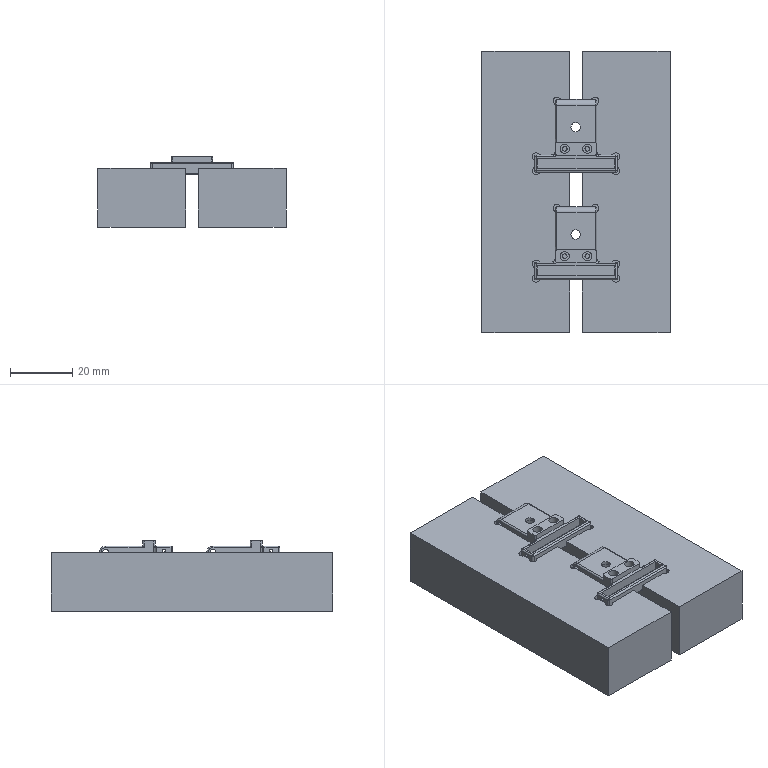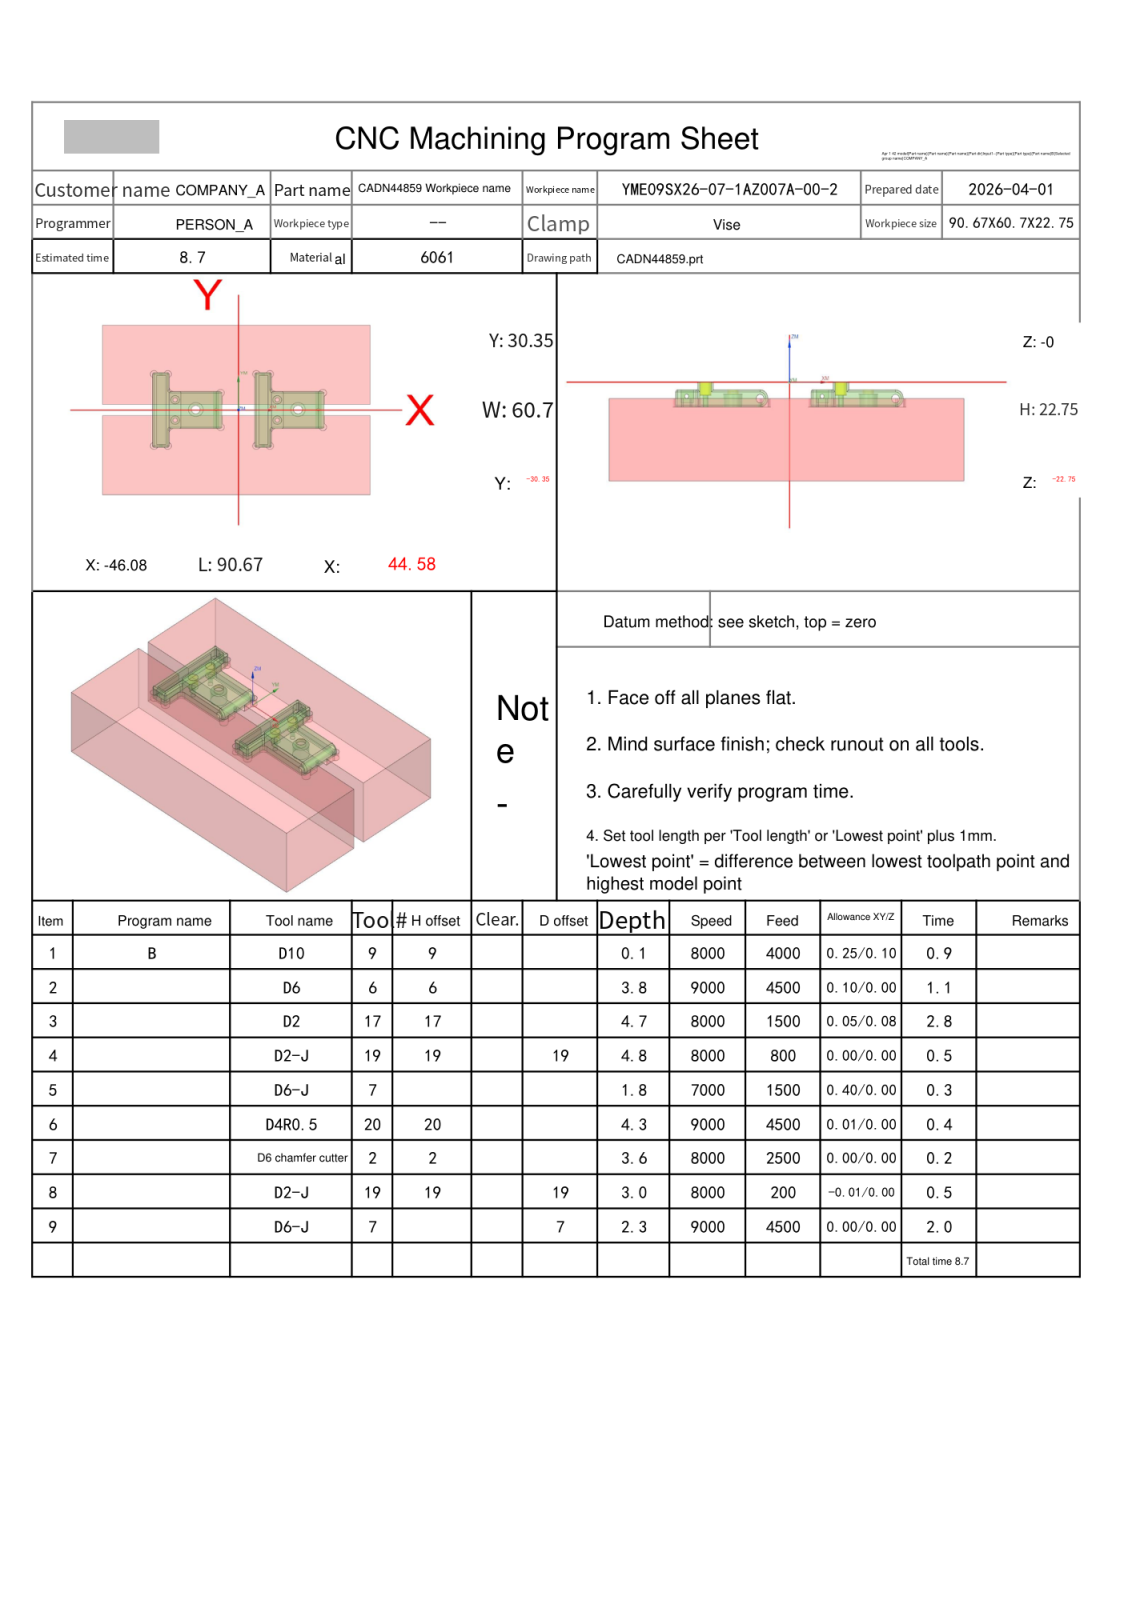NC program | NX | posted by the shop | part box 60.696 x 90.669 x 22.754 mm
Lines 3625 to 6042 of 6042, first 1914 of 2418 lines:
N7 T02 M06
(D6 chamfer cutter  D=6. R=0. H=02 ce=0.00 di=0.00)
G00 G90 G54 X-21.452 Y3.634 M03 S8000
G43 H02 Z20.
M08
G98 G82 X-21.452 Y3.634 Z-1. R1. F2500.
Y-3.634
X13.148
Y3.634
G80
G00 Z20.
G00 G90 X-14.452 Y.15 M03 S8000
Z20.
G98 G81 X-14.452 Y.15 Z-3.554 R1.246 F1000.
X20.148
G80
G00 Z20.
G00 G90 X-21.452 Y3.634 M03 S8000
Z20.
G98 G81 X-21.452 Y3.634 Z-1.8 R3. F1000.
Y-3.634
X13.148
Y3.634
G80
G00 Z20.
G00 G90 X10.121 Y-.386 M03 S6500
Z20.
Z.372
G01 Z-.999 F1500.
G03 X10.321 Y-.1 I-1.532 J1.286
G01 X10.351 Y-.054
X10.348 Y0.0
Y6.134
G02 X11.648 Y7.434 I1.3 J0.0
G01 X14.648
G02 X15.948 Y6.134 I0.0 J-1.3
G01 Y-6.134
G02 X14.648 Y-7.434 I-1.3 J0.0
G01 X11.648
G02 X10.348 Y-6.134 I0.0 J1.3
G01 Y0.0
X10.351 Y.054
X10.321 Y.1
G03 X10.121 Y.386 I-1.732 J-1.
G01 Z.372
G00 Z2.751
X12.736 Y3.108
Z.572
G01 Z-.999
G03 X13.045 Y2.947 I1.075 J1.687
G01 X13.094 Y2.924
X13.148 Y2.934
G03 X13.848 Y3.634 I0.0 J.7
X13.148 Y4.334 I-.7 J0.0
X12.448 Y3.634 I0.0 J-.7
X12.967 Y2.958 I.7 J0.0
G01 X13.148 Y2.934
X13.201 Y2.924
X13.25 Y2.947
G03 X13.56 Y3.108 I-.765 J1.848
G01 Z.572
G00 Z2.751
X12.736 Y-4.159
Z.572
G01 Z-.999
G03 X13.045 Y-4.32 I1.075 J1.687
G01 X13.094 Y-4.344
X13.148 Y-4.334
G03 X13.848 Y-3.634 I0.0 J.7
X13.148 Y-2.934 I-.7 J0.0
X12.448 Y-3.634 I0.0 J-.7
X12.967 Y-4.31 I.7 J0.0
G01 X13.148 Y-4.334
X13.201 Y-4.344
X13.25 Y-4.32
G03 X13.56 Y-4.159 I-.765 J1.848
G01 Z.572
G00 Z10.
X-18.426 Y.386
Z.372
G01 Z-.999
G03 X-18.625 Y.1 I1.532 J-1.286
G01 X-18.655 Y.054
X-18.652 Y0.0
Y-6.134
G02 X-19.952 Y-7.434 I-1.3 J0.0
G01 X-22.952
G02 X-24.252 Y-6.134 I0.0 J1.3
G01 Y6.134
G02 X-22.952 Y7.434 I1.3 J0.0
G01 X-19.952
G02 X-18.652 Y6.134 I0.0 J-1.3
G01 Y0.0
X-18.655 Y-.054
X-18.625 Y-.1
G03 X-18.426 Y-.386 I1.732 J1.
G01 Z.372
G00 Z2.751
X-21.864 Y3.108
Z.572
G01 Z-.999
G03 X-21.555 Y2.947 I1.075 J1.687
G01 X-21.506 Y2.924
X-21.452 Y2.934
G03 X-20.752 Y3.634 I0.0 J.7
X-21.452 Y4.334 I-.7 J0.0
X-22.152 Y3.634 I0.0 J-.7
X-21.633 Y2.958 I.7 J0.0
G01 X-21.452 Y2.934
X-21.399 Y2.924
X-21.35 Y2.947
G03 X-21.04 Y3.108 I-.765 J1.848
G01 Z.572
G00 Z2.751
X-21.864 Y-4.159
Z.572
G01 Z-.999
G03 X-21.555 Y-4.32 I1.075 J1.687
G01 X-21.506 Y-4.344
X-21.452 Y-4.334
G03 X-20.752 Y-3.634 I0.0 J.7
X-21.452 Y-2.934 I-.7 J0.0
X-22.152 Y-3.634 I0.0 J-.7
X-21.633 Y-4.31 I.7 J0.0
G01 X-21.452 Y-4.334
X-21.399 Y-4.344
X-21.35 Y-4.32
G03 X-21.04 Y-4.159 I-.765 J1.848
G01 Z.572
G00 Z10.
X-25.344 Y8.3
Z1.247
G01 Z-2.753
Y11.548
X-26.896
Y-11.548
X-25.344
Y-8.3
Z1.247
G00 Z10.
X-14.864 Y-.376
Z-1.182
G01 Z-2.753
G03 X-14.555 Y-.536 I1.075 J1.687
G01 X-14.506 Y-.56
X-14.452 Y-.55
G03 X-13.752 Y.15 I0.0 J.7
X-14.452 Y.85 I-.7 J0.0
X-15.152 Y.15 I0.0 J-.7
X-14.633 Y-.526 I.7 J0.0
G01 X-14.452 Y-.55
X-14.399 Y-.56
X-14.35 Y-.536
G03 X-14.04 Y-.376 I-.765 J1.848
G01 Z-1.182
G00 Z10.
X9.256 Y8.3
Z1.247
G01 Z-2.753
Y11.548
X7.704
Y0.0
Y-11.548
X9.256
Y-8.3
Z1.247
G00 Z10.
X19.736 Y-.376
Z-1.182
G01 Z-2.753
G03 X20.045 Y-.536 I1.075 J1.687
G01 X20.094 Y-.56
X20.148 Y-.55
G03 X20.848 Y.15 I0.0 J.7
X20.148 Y.85 I-.7 J0.0
X19.448 Y.15 I0.0 J-.7
X19.967 Y-.526 I.7 J0.0
G01 X20.148 Y-.55
X20.201 Y-.56
X20.25 Y-.536
G03 X20.56 Y-.376 I-.765 J1.848
G01 Z-1.182
G00 Z20.
G91 G28 Z0.0
M05
M09
G91 G28 Z0.0
M01
N8 T19 M06
(D2-J  D=2. R=0. H=19 ce=-0.01 di=0.00)
G00 G90 G54 X12.716 Y-3.825 M03 S8000
G43 H19 Z20.
M08
Z.5
G01 X12.737 Y-3.884 Z.497 F200.
X12.868 Y-4.025 Z.487
X13.043 Y-4.103 Z.477
X13.217 Y-4.11 Z.467
X13.363 Y-4.064 Z.459
X13.488 Y-3.974 Z.451
X13.578 Y-3.849 Z.443
X13.624 Y-3.703 Z.435
Y-3.565 Z.428
X13.578 Y-3.418 Z.42
X13.488 Y-3.294 Z.412
X13.363 Y-3.204 Z.404
X13.217 Y-3.158 Z.396
X13.079 Z.389
X12.932 Y-3.204 Z.381
X12.808 Y-3.294 Z.372
X12.718 Y-3.418 Z.364
X12.672 Y-3.565 Z.356
Y-3.703 Z.349
X12.737 Y-3.884 Z.339
X12.868 Y-4.025 Z.329
X13.043 Y-4.103 Z.319
X13.217 Y-4.11 Z.31
X13.363 Y-4.064 Z.302
X13.488 Y-3.974 Z.294
X13.578 Y-3.849 Z.286
X13.624 Y-3.703 Z.278
Y-3.565 Z.27
X13.578 Y-3.418 Z.262
X13.488 Y-3.294 Z.254
X13.363 Y-3.204 Z.246
X13.217 Y-3.158 Z.238
X13.079 Z.231
X12.932 Y-3.204 Z.223
X12.808 Y-3.294 Z.215
X12.718 Y-3.418 Z.207
X12.672 Y-3.565 Z.199
Y-3.703 Z.191
X12.737 Y-3.884 Z.181
X12.868 Y-4.025 Z.171
X13.043 Y-4.103 Z.161
X13.217 Y-4.11 Z.152
X13.363 Y-4.064 Z.144
X13.488 Y-3.974 Z.136
X13.578 Y-3.849 Z.128
X13.624 Y-3.703 Z.12
Y-3.565 Z.113
X13.578 Y-3.418 Z.105
X13.488 Y-3.294 Z.097
X13.363 Y-3.204 Z.089
X13.217 Y-3.158 Z.081
X13.079 Z.073
X12.932 Y-3.204 Z.065
X12.808 Y-3.294 Z.057
X12.718 Y-3.418 Z.049
X12.672 Y-3.565 Z.041
Y-3.703 Z.034
X12.737 Y-3.884 Z.024
X12.868 Y-4.025 Z.014
X13.043 Y-4.103 Z.004
X13.112 Y-4.108 Z0.0
G41 D19
X13.148 Y-4.144
G03 X13.658 Y-3.634 Z-.25 I0.0 J.51
X13.148 Y-3.124 Z-.5 I-.51 J0.0
X12.638 Y-3.634 Z-.75 I0.0 J-.51
X13.148 Y-4.144 Z-1. I.51 J0.0
X13.658 Y-3.634 Z-1.25 I0.0 J.51
X13.148 Y-3.124 Z-1.5 I-.51 J0.0
X12.638 Y-3.634 Z-1.75 I0.0 J-.51
X13.148 Y-4.144 Z-2. I.51 J0.0
X13.658 Y-3.634 Z-2.25 I0.0 J.51
X13.148 Y-3.124 Z-2.5 I-.51 J0.0
X12.638 Y-3.634 Z-2.75 I0.0 J-.51
X13.148 Y-4.144 Z-3. I.51 J0.0
X13.658 Y-3.634 I0.0 J.51
X13.148 Y-3.124 I-.51 J0.0
X12.638 Y-3.634 I0.0 J-.51
X13.148 Y-4.144 I.51 J0.0
X13.508 Y-3.995 I0.0 J.51
G01 X13.526 Y-3.974
Y-3.945
X13.508 Y-3.924
G40 X13.473 Y-3.889
Z-2.
G00 Z20.
X13.58 Y3.825
Z.5
G01 X13.559 Y3.884 Z.497
X13.428 Y4.025 Z.487
X13.252 Y4.103 Z.477
X13.079 Y4.11 Z.467
X12.932 Y4.064 Z.459
X12.808 Y3.974 Z.451
X12.718 Y3.849 Z.443
X12.672 Y3.703 Z.435
Y3.565 Z.428
X12.718 Y3.418 Z.42
X12.808 Y3.294 Z.412
X12.932 Y3.204 Z.404
X13.079 Y3.158 Z.396
X13.217 Z.389
X13.363 Y3.204 Z.381
X13.488 Y3.294 Z.372
X13.578 Y3.418 Z.364
X13.624 Y3.565 Z.356
Y3.703 Z.349
X13.559 Y3.884 Z.339
X13.428 Y4.025 Z.329
X13.252 Y4.103 Z.319
X13.079 Y4.11 Z.31
X12.932 Y4.064 Z.302
X12.808 Y3.974 Z.294
X12.718 Y3.849 Z.286
X12.672 Y3.703 Z.278
Y3.565 Z.27
X12.718 Y3.418 Z.262
X12.808 Y3.294 Z.254
X12.932 Y3.204 Z.246
X13.079 Y3.158 Z.238
X13.217 Z.231
X13.363 Y3.204 Z.223
X13.488 Y3.294 Z.215
X13.578 Y3.418 Z.207
X13.624 Y3.565 Z.199
Y3.703 Z.191
X13.559 Y3.884 Z.181
X13.428 Y4.025 Z.171
X13.252 Y4.103 Z.161
X13.079 Y4.11 Z.152
X12.932 Y4.064 Z.144
X12.808 Y3.974 Z.136
X12.718 Y3.849 Z.128
X12.672 Y3.703 Z.12
Y3.565 Z.113
X12.718 Y3.418 Z.105
X12.808 Y3.294 Z.097
X12.932 Y3.204 Z.089
X13.079 Y3.158 Z.081
X13.217 Z.073
X13.363 Y3.204 Z.065
X13.488 Y3.294 Z.057
X13.578 Y3.418 Z.049
X13.624 Y3.565 Z.041
Y3.703 Z.034
X13.559 Y3.884 Z.024
X13.428 Y4.025 Z.014
X13.252 Y4.103 Z.004
X13.183 Y4.108 Z0.0
G41 D19
X13.148 Y4.144
G03 X12.638 Y3.634 Z-.25 I0.0 J-.51
X13.148 Y3.124 Z-.5 I.51 J0.0
X13.658 Y3.634 Z-.75 I0.0 J.51
X13.148 Y4.144 Z-1. I-.51 J0.0
X12.638 Y3.634 Z-1.25 I0.0 J-.51
X13.148 Y3.124 Z-1.5 I.51 J0.0
X13.658 Y3.634 Z-1.75 I0.0 J.51
X13.148 Y4.144 Z-2. I-.51 J0.0
X12.638 Y3.634 Z-2.25 I0.0 J-.51
X13.148 Y3.124 Z-2.5 I.51 J0.0
X13.658 Y3.634 Z-2.75 I0.0 J.51
X13.148 Y4.144 Z-3. I-.51 J0.0
X12.638 Y3.634 I0.0 J-.51
X13.148 Y3.124 I.51 J0.0
X13.658 Y3.634 I0.0 J.51
X13.148 Y4.144 I-.51 J0.0
X12.787 Y3.995 I0.0 J-.51
G01 X12.77 Y3.974
Y3.945
X12.787 Y3.924
G40 X12.823 Y3.889
Z-2.
G00 Z20.
X-21.643 Y4.066
Z.5
G01 X-21.702 Y4.045 Z.497
X-21.843 Y3.914 Z.487
X-21.922 Y3.738 Z.477
X-21.928 Y3.565 Z.467
X-21.882 Y3.418 Z.459
X-21.792 Y3.294 Z.451
X-21.668 Y3.204 Z.443
X-21.521 Y3.158 Z.435
X-21.383 Z.428
X-21.237 Y3.204 Z.42
X-21.112 Y3.294 Z.412
X-21.022 Y3.418 Z.404
X-20.976 Y3.565 Z.396
Y3.703 Z.389
X-21.022 Y3.849 Z.381
X-21.112 Y3.974 Z.372
X-21.237 Y4.064 Z.364
X-21.383 Y4.11 Z.356
X-21.521 Z.349
X-21.702 Y4.045 Z.339
X-21.843 Y3.914 Z.329
X-21.922 Y3.738 Z.319
X-21.928 Y3.565 Z.31
X-21.882 Y3.418 Z.302
X-21.792 Y3.294 Z.294
X-21.668 Y3.204 Z.286
X-21.521 Y3.158 Z.278
X-21.383 Z.27
X-21.237 Y3.204 Z.262
X-21.112 Y3.294 Z.254
X-21.022 Y3.418 Z.246
X-20.976 Y3.565 Z.238
Y3.703 Z.231
X-21.022 Y3.849 Z.223
X-21.112 Y3.974 Z.215
X-21.237 Y4.064 Z.207
X-21.383 Y4.11 Z.199
X-21.521 Z.191
X-21.702 Y4.045 Z.181
X-21.843 Y3.914 Z.171
X-21.922 Y3.738 Z.161
X-21.928 Y3.565 Z.152
X-21.882 Y3.418 Z.144
X-21.792 Y3.294 Z.136
X-21.668 Y3.204 Z.128
X-21.521 Y3.158 Z.12
X-21.383 Z.113
X-21.237 Y3.204 Z.105
X-21.112 Y3.294 Z.097
X-21.022 Y3.418 Z.089
X-20.976 Y3.565 Z.081
Y3.703 Z.073
X-21.022 Y3.849 Z.065
X-21.112 Y3.974 Z.057
X-21.237 Y4.064 Z.049
X-21.383 Y4.11 Z.041
X-21.521 Z.034
X-21.702 Y4.045 Z.024
X-21.843 Y3.914 Z.014
X-21.922 Y3.738 Z.004
X-21.927 Y3.669 Z0.0
G41 D19
X-21.962 Y3.634
G03 X-21.452 Y3.124 Z-.25 I.51 J0.0
X-20.942 Y3.634 Z-.5 I0.0 J.51
X-21.452 Y4.144 Z-.75 I-.51 J0.0
X-21.962 Y3.634 Z-1. I0.0 J-.51
X-21.452 Y3.124 Z-1.25 I.51 J0.0
X-20.942 Y3.634 Z-1.5 I0.0 J.51
X-21.452 Y4.144 Z-1.75 I-.51 J0.0
X-21.962 Y3.634 Z-2. I0.0 J-.51
X-21.452 Y3.124 Z-2.25 I.51 J0.0
X-20.942 Y3.634 Z-2.5 I0.0 J.51
X-21.452 Y4.144 Z-2.75 I-.51 J0.0
X-21.962 Y3.634 Z-3. I0.0 J-.51
X-21.452 Y3.124 I.51 J0.0
X-20.942 Y3.634 I0.0 J.51
X-21.452 Y4.144 I-.51 J0.0
X-21.962 Y3.634 I0.0 J-.51
X-21.813 Y3.274 I.51 J0.0
G01 X-21.792 Y3.256
X-21.764
X-21.743 Y3.274
G40 X-21.707 Y3.309
Z-2.
G00 Z20.
X-21.643 Y-3.202
Z.5
G01 X-21.702 Y-3.223 Z.497
X-21.843 Y-3.354 Z.487
X-21.922 Y-3.53 Z.477
X-21.928 Y-3.703 Z.467
X-21.882 Y-3.849 Z.459
X-21.792 Y-3.974 Z.451
X-21.668 Y-4.064 Z.443
X-21.521 Y-4.11 Z.435
X-21.383 Z.428
X-21.237 Y-4.064 Z.42
X-21.112 Y-3.974 Z.412
X-21.022 Y-3.849 Z.404
X-20.976 Y-3.703 Z.396
Y-3.565 Z.389
X-21.022 Y-3.418 Z.381
X-21.112 Y-3.294 Z.372
X-21.237 Y-3.204 Z.364
X-21.383 Y-3.158 Z.356
X-21.521 Z.349
X-21.702 Y-3.223 Z.339
X-21.843 Y-3.354 Z.329
X-21.922 Y-3.53 Z.319
X-21.928 Y-3.703 Z.31
X-21.882 Y-3.849 Z.302
X-21.792 Y-3.974 Z.294
X-21.668 Y-4.064 Z.286
X-21.521 Y-4.11 Z.278
X-21.383 Z.27
X-21.237 Y-4.064 Z.262
X-21.112 Y-3.974 Z.254
X-21.022 Y-3.849 Z.246
X-20.976 Y-3.703 Z.238
Y-3.565 Z.231
X-21.022 Y-3.418 Z.223
X-21.112 Y-3.294 Z.215
X-21.237 Y-3.204 Z.207
X-21.383 Y-3.158 Z.199
X-21.521 Z.191
X-21.702 Y-3.223 Z.181
X-21.843 Y-3.354 Z.171
X-21.922 Y-3.53 Z.161
X-21.928 Y-3.703 Z.152
X-21.882 Y-3.849 Z.144
X-21.792 Y-3.974 Z.136
X-21.668 Y-4.064 Z.128
X-21.521 Y-4.11 Z.12
X-21.383 Z.113
X-21.237 Y-4.064 Z.105
X-21.112 Y-3.974 Z.097
X-21.022 Y-3.849 Z.089
X-20.976 Y-3.703 Z.081
Y-3.565 Z.073
X-21.022 Y-3.418 Z.065
X-21.112 Y-3.294 Z.057
X-21.237 Y-3.204 Z.049
X-21.383 Y-3.158 Z.041
X-21.521 Z.034
X-21.702 Y-3.223 Z.024
X-21.843 Y-3.354 Z.014
X-21.922 Y-3.53 Z.004
X-21.927 Y-3.598 Z0.0
G41 D19
X-21.962 Y-3.634
G03 X-21.452 Y-4.144 Z-.25 I.51 J0.0
X-20.942 Y-3.634 Z-.5 I0.0 J.51
X-21.452 Y-3.124 Z-.75 I-.51 J0.0
X-21.962 Y-3.634 Z-1. I0.0 J-.51
X-21.452 Y-4.144 Z-1.25 I.51 J0.0
X-20.942 Y-3.634 Z-1.5 I0.0 J.51
X-21.452 Y-3.124 Z-1.75 I-.51 J0.0
X-21.962 Y-3.634 Z-2. I0.0 J-.51
X-21.452 Y-4.144 Z-2.25 I.51 J0.0
X-20.942 Y-3.634 Z-2.5 I0.0 J.51
X-21.452 Y-3.124 Z-2.75 I-.51 J0.0
X-21.962 Y-3.634 Z-3. I0.0 J-.51
X-21.452 Y-4.144 I.51 J0.0
X-20.942 Y-3.634 I0.0 J.51
X-21.452 Y-3.124 I-.51 J0.0
X-21.962 Y-3.634 I0.0 J-.51
X-21.813 Y-3.994 I.51 J0.0
G01 X-21.792 Y-4.012
X-21.764
X-21.743 Y-3.994
G40 X-21.707 Y-3.959
Z-2.
G00 Z20.
G91 G28 Z0.0
M05
M09
G91 G28 Z0.0
M01
N9 T07 M06
(D6-J  D=6. R=0. H=00 ce=0.00 di=0.00)
G00 G90 G54 X13.748 Y10.734 M03 S8000
G43 H00 Z6.95
M08
Z-.754
G01 Z-1.754 F1000.
G41 D07
Y10.534
G03 X14.648 Y9.634 I.9 J0.0
G02 X18.148 Y6.134 I0.0 J-3.5
G01 Y6.131
Y-6.129
Y-6.134
G02 X14.648 Y-9.634 I-3.5 J0.0
G03 X13.748 Y-10.534 I0.0 J-.9
G01 G40 Y-10.734
Z-.754
G00 Z6.95
X12.548
Z-.754
G01 Z-1.754
G41 D07
Y-10.534
G03 X11.648 Y-9.634 I-.9 J0.0
G02 X8.148 Y-6.134 I0.0 J3.5
G01 Y6.134
G02 X11.648 Y9.634 I3.5 J0.0
G03 X12.548 Y10.534 I0.0 J.9
G01 G40 Y10.734
Z-.754
G00 Z6.95
X-20.852
Z-.754
G01 Z-1.754
G41 D07
Y10.534
G03 X-19.952 Y9.634 I.9 J0.0
G02 X-16.452 Y6.134 I0.0 J-3.5
G01 Y6.131
Y-6.129
Y-6.134
G02 X-19.952 Y-9.634 I-3.5 J0.0
G03 X-20.852 Y-10.534 I0.0 J-.9
G01 G40 Y-10.734
Z-.754
G00 Z6.95
X-22.052
Z-.754
G01 Z-1.754
G41 D07
Y-10.534
G03 X-22.952 Y-9.634 I-.9 J0.0
G02 X-26.452 Y-6.134 I0.0 J3.5
G01 Y6.134
G02 X-22.952 Y9.634 I3.5 J0.0
G03 X-22.052 Y10.534 I0.0 J.9
G01 G40 Y10.734
Z-.754
G00 Z6.95
G00 G90 X-3.703 Y-11.541 M03 S9000
Z11.95
Z-1.262
G01 Z-1.762 F4500.
G03 X-6.415 Y-9.176 I-2.934 J-.627
X-6.741 Y-9.164 I-.326 J-4.399
X-7.515 Y-9.233 I0.0 J-4.411
G01 X-18.304
X-18.342 Y-9.253 Z-1.766
X-7.515
G02 X-6.724 Y-9.189 I.792 J-4.853
X-6.415 Y-9.198 I0.0 J-4.917
G01 X-6.414 Y-9.221 Z-1.77
G03 X-6.696 Y-9.214 I-.282 J-6.068
X-7.515 Y-9.27 I0.0 J-6.074
G01 X-18.375
X-18.405 Y-9.285 Z-1.774
X-7.515
G02 X-6.672 Y-9.239 I.844 J-7.802
X-6.414 Y-9.243 I0.0 J-7.848
G01 X-6.413 Y-9.27 Z-1.779
G03 X-7.515 Y-9.3 I1.192 J-63.284
G01 X-18.437
X-18.467 Y-9.314 Z-1.784
X-7.515
X-6.412 Y-9.296
X-6.414 Y-9.312 Z-1.787
Y-9.313 Z-1.789
X-6.6
G03 X-7.515 Y-9.329 I0.0 J-26.271
G01 X-18.499
X-18.53 Y-9.343 Z-1.795
X-7.515
G02 X-6.603 Y-9.325 I.913 J-23.879
G01 X-6.414 Y-9.326
Y-9.338 Z-1.798
Y-9.34 Z-1.802
G03 X-7.515 Y-9.357 I.605 J-74.86
G01 X-18.561
X-18.594 Y-9.37 Z-1.808
X-7.515
G02 X-6.413 Y-9.354 I5.167 J-313.246
G01 Y-9.368 Z-1.812
Y-9.369 Z-1.815
X-7.515 Y-9.384
X-18.626
X-18.658 Y-9.397 Z-1.823
X-7.515
X-6.413 Y-9.385
X-6.414 Y-9.396 Z-1.827
Y-9.398 Z-1.831
X-7.515 Y-9.41
X-18.692
X-18.725 Y-9.422 Z-1.839
X-7.515
G02 X-6.549 Y-9.409 I.966 J-35.239
G01 X-6.414
Y-9.42 Z-1.843
Y-9.421 Z-1.847
X-6.547
G03 X-7.515 Y-9.435 I0.0 J-33.728
G01 X-18.759
X-18.777 Y-9.441 Z-1.856
X-7.515
G02 X-6.539 Y-9.427 I.977 J-34.327
G01 X-6.415
Y-9.445 Z-1.861
Y-9.446 Z-1.866
X-7.515 Y-9.459
X-18.828
X-18.859 Y-9.469 Z-1.875
X-7.515
X-6.415 Y-9.458
X-6.416 Y-9.47 Z-1.881
Y-9.473 Z-1.886
X-7.515 Y-9.482
X-18.898
X-18.934 Y-9.493 Z-1.896
X-7.515
X-6.414 Y-9.486
Y-9.495 Z-1.907
X-7.515 Y-9.503
X-18.969
X-19.006 Y-9.514 Z-1.918
X-7.515
G02 X-6.723 Y-9.504 I.793 J-30.792
X-6.414 Y-9.505 I0.0 J-30.803
G01 Y-9.513 Z-1.929
G03 X-6.725 Y-9.511 I-.311 J-30.346
X-7.515 Y-9.522 I0.0 J-30.347
G01 X-19.034
X-19.079 Y-9.533 Z-1.941
X-7.515
G02 X-6.728 Y-9.524 I.787 J-32.489
X-6.414 Y-9.525 I0.0 J-32.498
G01 Y-9.532 Z-1.947
Y-9.536 Z-1.952
X-7.515 Y-9.543
X-19.116
X-19.153 Y-9.552 Z-1.965
X-7.515
X-6.414 Y-9.547
Y-9.548 Z-1.971
Y-9.557 Z-1.977
X-7.515 Y-9.56
X-19.19
X-19.228 Y-9.568 Z-1.99
X-7.515
X-6.414 Y-9.565
Y-9.572 Z-2.003
X-7.515 Y-9.576
X-19.266
X-19.304 Y-9.583 Z-2.016
X-7.515
X-6.414 Y-9.579
Y-9.586 Z-2.029
X-7.515 Y-9.59
X-19.342
X-19.381 Y-9.597 Z-2.043
X-7.515
X-6.414 Y-9.593
Y-9.6 Z-2.056
X-7.515 Y-9.603
X-19.419
X-19.458 Y-9.609 Z-2.07
X-7.515
X-6.414 Y-9.603
Y-9.607 Z-2.084
X-7.515 Y-9.614
X-19.497
X-19.536 Y-9.619 Z-2.099
X-7.515
X-6.414 Y-9.611
Y-9.614 Z-2.113
X-7.515 Y-9.624
X-19.576
X-19.615 Y-9.628 Z-2.128
X-7.515
X-6.42 Y-9.617
X-6.414 Y-9.618
Y-9.622 Z-2.142
X-6.42 Y-9.62
X-7.515 Y-9.631
X-19.654
X-19.694 Y-9.634 Z-2.157
X-7.515
X-6.42 Y-9.623
X-6.414 Y-9.626
Y-9.63 Z-2.172
X-6.42 Y-9.627
X-7.515 Y-9.637
X-19.733
X-19.773 Y-9.639 Z-2.186
X-7.515
X-6.42 Y-9.63
X-6.414 Y-9.633
Y-9.635 Z-2.201
X-7.515 Y-9.641
X-19.813
X-19.852 Y-9.642 Z-2.216
X-7.515
X-6.42 Y-9.637
X-6.414 Y-9.638
Y-9.641 Z-2.231
X-19.852 Y-9.643
X-19.892
X-20.03 Y-9.644 Z-2.237
X-20.169 Z-2.243
X-20.31 Z-2.248
X-20.442 Y-9.654 Z-2.254
X-20.432 Y-9.644
X-19.93
X-19.87 Y-9.643
X-6.414
G00 Z11.95
X-15.305 Y12.233
Z-1.262
G01 Z-1.762
G03 X-18.304 Y9.233 I0.0 J-3.
G01 X-7.515
X-6.863 Y9.178
X-6.418 Y9.186
X-6.419 Y9.208 Z-1.766
X-6.863 Y9.2
G03 X-7.515 Y9.253 I-.86 J-6.625
G01 X-18.342
X-18.375 Y9.27 Z-1.77
X-7.515
G03 X-6.627 Y9.226 I.889 J9.11
X-6.418 Y9.229 I0.0 J9.153
G01 X-6.417 Y9.25 Z-1.774
G02 X-6.631 Y9.248 I-.213 J10.606
X-7.515 Y9.285 I0.0 J10.608
G01 X-18.405
X-18.437 Y9.3 Z-1.779
X-7.515
X-6.416 Y9.274
X-6.414 Y9.295 Z-1.781
X-6.413 Y9.299 Z-1.784
X-7.515 Y9.314
X-18.467
X-18.499 Y9.329 Z-1.789
X-7.515
G03 X-6.6 Y9.313 I.916 J26.601
G01 X-6.414 Y9.314
Y9.323 Z-1.792
Y9.326 Z-1.795
X-6.604 Y9.325
G02 X-7.515 Y9.343 I0.0 J23.966
G01 X-18.53
X-18.561 Y9.357 Z-1.802
X-7.515
G03 X-6.593 Y9.339 I.923 J24.065
G01 X-6.414 Y9.34
X-6.413 Y9.352 Z-1.805
Y9.354 Z-1.808
X-6.563
G02 X-7.515 Y9.37 I0.0 J27.089
G01 X-18.594
X-18.626 Y9.384 Z-1.815
X-7.515
X-6.413 Y9.369
Y9.382 Z-1.819
Y9.385 Z-1.823
X-7.515 Y9.397
X-18.658
X-18.692 Y9.41 Z-1.831
X-7.515
G03 X-6.534 Y9.398 I.981 J40.461
G01 X-6.414
Y9.407 Z-1.835
Y9.409 Z-1.839
X-6.553
G02 X-7.515 Y9.422 I0.0 J34.718
G01 X-18.725
X-18.759 Y9.435 Z-1.847
X-7.515
G03 X-6.548 Y9.421 I.967 J33.574
G01 X-6.414
X-6.415 Y9.427 Z-1.856
X-6.539
G02 X-7.515 Y9.441 I0.0 J34.388
G01 X-18.777
X-18.828 Y9.459 Z-1.866
X-7.515
G03 X-6.46 Y9.446 I1.056 J44.602
G01 X-6.415
Y9.459 Z-1.871
Y9.458 Z-1.875
X-7.515 Y9.469
X-18.859
X-18.898 Y9.482 Z-1.886
X-7.515
X-6.416 Y9.474
X-6.415 Y9.483 Z-1.891
X-6.414 Y9.486 Z-1.896
X-7.515 Y9.493
X-18.934
X-18.969 Y9.503 Z-1.907
X-7.515
X-6.414 Y9.495
Y9.505 Z-1.918
G02 X-6.722 Y9.504 I-.308 J31.247
X-7.515 Y9.514 I0.0 J31.249
G01 X-19.006
X-19.034 Y9.522 Z-1.929
X-7.515
G03 X-6.725 Y9.512 I.791 J30.705
X-6.414 Y9.513 I0.0 J30.715
G01 Y9.522 Z-1.935
Y9.525 Z-1.941
X-6.517
X-7.515 Y9.533
X-19.079
X-19.116 Y9.543 Z-1.952
X-7.515
X-6.414 Y9.536
Y9.54 Z-1.959
Y9.547 Z-1.965
X-6.517 Y9.546
X-7.515 Y9.552
X-19.153
X-19.19 Y9.56 Z-1.977
X-7.515
X-6.517 Y9.557
X-6.414
Y9.565 Z-1.99
X-7.515 Y9.568
X-19.228
X-19.266 Y9.576 Z-2.003
X-7.515
X-6.414 Y9.572
Y9.579 Z-2.016
X-7.515 Y9.583
X-19.304
X-19.342 Y9.59 Z-2.029
X-7.515
X-6.414 Y9.586
Y9.593 Z-2.043
X-7.515 Y9.597
X-19.381
X-19.419 Y9.603 Z-2.056
X-7.515
X-6.414 Y9.6
Y9.603 Z-2.07
X-7.515 Y9.609
X-19.458
X-19.497 Y9.614 Z-2.084
X-7.515
X-6.517 Y9.607
X-6.414
Y9.611 Z-2.099
X-7.515 Y9.619
X-19.536
X-19.576 Y9.624 Z-2.113
X-7.515
X-6.414 Y9.614
Y9.618 Z-2.128
X-6.42 Y9.617
X-7.515 Y9.628
X-19.615
X-19.654 Y9.631 Z-2.142
X-7.515
X-6.42 Y9.62
X-6.414 Y9.622
Y9.626 Z-2.157
X-6.42 Y9.623
X-7.515 Y9.634
X-19.856
X-19.871 Y9.637 Z-2.172
X-7.515
X-6.42 Y9.627
X-6.414 Y9.63
Y9.633 Z-2.186
X-6.42 Y9.63
X-7.515 Y9.639
X-19.885
X-20.017 Y9.644 Z-2.19
X-20.149 Z-2.194
X-20.281 Z-2.198
X-20.413 Z-2.201
X-19.9 Y9.641
X-7.515
X-6.414 Y9.635
Y9.638 Z-2.216
X-7.515 Y9.642
X-19.915
X-20.413 Y9.644
X-20.443 Y9.651 Z-2.231
X-20.352 Y9.643
X-18.968
X-18.929
X-7.209 Y9.641
X-6.414
Y9.643 Z-2.254
X-18.929 Y9.644
X-18.968
X-20.352 Y9.643
X-20.442 Y9.651
G00 Z11.95
X30.887 Y-11.574
Z-1.262
G01 Z-1.762
G03 X28.185 Y-9.176 I-2.941 J-.593
X27.849 Y-9.163 I-.335 J-4.205
X27.085 Y-9.233 I0.0 J-4.218
G01 X16.296
X16.258 Y-9.253 Z-1.766
X27.085
G02 X27.411 Y-9.201 I.33 J-1.036
G01 X28.185 Y-9.198
Y-9.221 Z-1.77
G03 X27.9 Y-9.214 I-.286 J-5.971
X27.085 Y-9.27 I0.0 J-5.978
G01 X16.225
X16.195 Y-9.285 Z-1.774
X27.085
G02 X27.926 Y-9.239 I.842 J-7.74
X28.186 Y-9.243 I0.0 J-7.785
G01 X28.187 Y-9.27 Z-1.779
G03 X27.085 Y-9.3 I.864 J-51.281
G01 X16.163
X16.133 Y-9.314 Z-1.784
X27.085
X28.188 Y-9.296
X28.186 Y-9.312 Z-1.787
Y-9.313 Z-1.789
X27.998
G03 X27.085 Y-9.329 I0.0 J-26.077
G01 X16.101
X16.07 Y-9.343 Z-1.795
X27.085
G02 X27.995 Y-9.325 I.911 J-23.702
G01 X28.186 Y-9.326
Y-9.338 Z-1.798
Y-9.339 Z-1.802
X28.008
G03 X27.085 Y-9.357 I0.0 J-24.073
G01 X16.039
X16.006 Y-9.37 Z-1.808
X27.085
G02 X28.186 Y-9.354 I4.97 J-299.214
G01 Y-9.368 Z-1.812
Y-9.369 Z-1.815
X27.085 Y-9.384
X15.974
X15.942 Y-9.397 Z-1.823
X27.085
X28.186 Y-9.385
Y-9.396 Z-1.827
Y-9.398 Z-1.831
X27.085 Y-9.41
X15.908
X15.875 Y-9.422 Z-1.839
X27.085
G02 X28.049 Y-9.409 I.965 J-35.024
G01 X28.185
Y-9.42 Z-1.843
Y-9.421 Z-1.847
X28.051
G03 X27.085 Y-9.435 I0.0 J-33.531
G01 X15.841
X15.823 Y-9.441 Z-1.856
X27.085
G02 X28.06 Y-9.427 I.975 J-34.134
G01 X28.185
Y-9.445 Z-1.861
Y-9.446 Z-1.866
X27.085 Y-9.459
X15.772
X15.741 Y-9.469 Z-1.875
X27.085
X28.185 Y-9.458
X28.184 Y-9.47 Z-1.881
Y-9.473 Z-1.886
X27.085 Y-9.482
X15.702
X15.666 Y-9.493 Z-1.896
X27.085
X28.184 Y-9.486
Y-9.495 Z-1.907
G03 X27.085 Y-9.503 I3.539 J-556.894
G01 X15.631
X15.594 Y-9.514 Z-1.918
X27.085
G02 X27.874 Y-9.504 I.789 J-30.37
X28.184 Y-9.505 I0.0 J-30.38
G01 Y-9.513 Z-1.929
G03 X27.871 Y-9.511 I-.313 J-29.934
X27.085 Y-9.522 I0.0 J-29.936
G01 X15.566
X15.521 Y-9.533 Z-1.941
X27.085
G02 X27.868 Y-9.524 I.784 J-32.059
X28.184 Y-9.525 I0.0 J-32.068
G01 Y-9.532 Z-1.947
Y-9.536 Z-1.952
X27.085 Y-9.543
X15.484
X15.447 Y-9.552 Z-1.965
X27.085
X28.184 Y-9.547
Y-9.548 Z-1.971
Y-9.557 Z-1.977
X27.085 Y-9.56
X15.41
X15.372 Y-9.568 Z-1.99
X27.085
X28.184 Y-9.565
Y-9.572 Z-2.003
X27.085 Y-9.576
X15.334
X15.296 Y-9.583 Z-2.016
X27.085
X28.184 Y-9.579
Y-9.586 Z-2.029
X27.085 Y-9.59
X15.258
X15.219 Y-9.597 Z-2.043
X27.085
X28.184 Y-9.593
Y-9.6 Z-2.056
X27.085 Y-9.603
X15.181
X15.142 Y-9.609 Z-2.07
X27.085
X28.184 Y-9.603
Y-9.607 Z-2.084
X27.085 Y-9.614
X15.103
X15.064 Y-9.619 Z-2.099
X27.085
X28.184 Y-9.611
Y-9.614 Z-2.113
X27.085 Y-9.624
X15.024
X14.985 Y-9.628 Z-2.128
X27.085
X28.179 Y-9.617
X28.184 Y-9.618
Y-9.622 Z-2.142
X28.179 Y-9.62
X27.085 Y-9.631
X14.946
X14.906 Y-9.634 Z-2.157
X27.085
X28.179 Y-9.623
X28.184 Y-9.626
Y-9.63 Z-2.172
X28.179 Y-9.627
X27.085 Y-9.637
X14.867
X14.827 Y-9.639 Z-2.186
X27.085
X28.179 Y-9.63
X28.184 Y-9.633
Y-9.635 Z-2.201
X27.085 Y-9.641
X14.787
X14.748 Y-9.642 Z-2.216
X27.085
X28.184 Y-9.638
Y-9.641 Z-2.231
X14.742 Y-9.643
X14.708
X14.569 Y-9.644 Z-2.237
X14.427 Z-2.243
X14.272 Z-2.248
X14.158 Y-9.657 Z-2.254
X14.159 Y-9.644
X14.668
X14.73 Y-9.643
X28.184
G00 Z11.95
X19.295 Y12.233
Z-1.262
G01 Z-1.762
G03 X16.296 Y9.233 I0.0 J-3.
G01 X27.085
X27.725 Y9.178
X28.182 Y9.187
X28.181 Y9.209 Z-1.766
X27.725 Y9.2
G03 X27.085 Y9.253 I-.869 J-6.686
G01 X16.258
X16.225 Y9.27 Z-1.77
X27.085
G03 X27.945 Y9.226 I.86 J8.53
X28.181 Y9.23 I0.0 J8.573
G01 X28.182 Y9.25 Z-1.774
G02 X27.944 Y9.247 I-.238 J9.978
X27.085 Y9.285 I0.0 J9.981
G01 X16.195
X16.163 Y9.3 Z-1.779
X27.085
X28.184 Y9.274
X28.186 Y9.295 Z-1.781
Y9.299 Z-1.784
X27.085 Y9.314
X16.133
X16.101 Y9.329 Z-1.789
X27.085
G03 X27.998 Y9.313 I.914 J26.403
G01 X28.186 Y9.314
Y9.323 Z-1.792
Y9.326 Z-1.795
X27.994 Y9.325
G02 X27.085 Y9.343 I0.0 J23.782
G01 X16.07
X16.039 Y9.357 Z-1.802
X27.085
G03 X28.005 Y9.339 I.92 J23.878
G01 X28.186
Y9.352 Z-1.805
Y9.354 Z-1.808
X28.035 Y9.353
G02 X27.085 Y9.37 I0.0 J26.906
G01 X16.006
X15.974 Y9.384 Z-1.815
X27.085
X28.186 Y9.369
Y9.382 Z-1.819
Y9.385 Z-1.823
X27.085 Y9.397
X15.942
X15.908 Y9.41 Z-1.831
X27.085
G03 X28.064 Y9.398 I.98 J40.199
G01 X28.186
X28.185 Y9.407 Z-1.835
Y9.409 Z-1.839
X28.046
G02 X27.085 Y9.422 I0.0 J34.507
G01 X15.875
X15.841 Y9.435 Z-1.847
X27.085
G03 X28.05 Y9.421 I.966 J33.378
G01 X28.185
Y9.427 Z-1.856
X28.06
G02 X27.085 Y9.441 I0.0 J34.196
G01 X15.823
X15.772 Y9.459 Z-1.866
X27.085
G03 X28.14 Y9.446 I1.055 J44.433
G01 X28.185
Y9.459 Z-1.871
Y9.458 Z-1.875
X27.085 Y9.469
X15.741
X15.702 Y9.482 Z-1.886
X27.085
X28.184 Y9.474
Y9.486 Z-1.896
X27.085 Y9.493
X15.666
X15.631 Y9.503 Z-1.907
X27.085
X28.184 Y9.495
Y9.505 Z-1.918
G02 X27.875 Y9.504 I-.31 J30.9
X27.085 Y9.514 I0.0 J30.902
G01 X15.594
X15.566 Y9.522 Z-1.929
X27.085
G03 X27.872 Y9.511 I.787 J30.365
X28.184 Y9.513 I0.0 J30.375
G01 Y9.522 Z-1.935
Y9.525 Z-1.941
X28.071
X27.085 Y9.533
X15.521
X15.484 Y9.543 Z-1.952
X27.085
X28.184 Y9.536
Y9.54 Z-1.959
Y9.547 Z-1.965
X28.071 Y9.546
X27.085 Y9.552
X15.447
X15.41 Y9.56 Z-1.977
X27.085
X28.071 Y9.557
X28.184
Y9.565 Z-1.99
X27.085 Y9.568
X15.372
X15.334 Y9.576 Z-2.003
X27.085
X28.184 Y9.572
Y9.579 Z-2.016
X27.085 Y9.583
X15.296
X15.258 Y9.59 Z-2.029
X27.085
X28.184 Y9.586
Y9.593 Z-2.043
X27.085 Y9.597
X15.219
X15.181 Y9.603 Z-2.056
X27.085
X28.184 Y9.6
Y9.603 Z-2.07
X27.085 Y9.609
X15.142
X15.103 Y9.614 Z-2.084
X27.085
X28.071 Y9.607
X28.184
Y9.611 Z-2.099
X27.085 Y9.619
X15.064
X15.024 Y9.624 Z-2.113
X27.085
X28.184 Y9.614
Y9.618 Z-2.128
X28.179 Y9.617
X27.085 Y9.628
X14.985
X14.946 Y9.631 Z-2.142
X27.085
X28.179 Y9.62
X28.184 Y9.622
Y9.626 Z-2.157
X28.179 Y9.623
X27.085 Y9.634
X14.744
X14.729 Y9.637 Z-2.172
X27.085
X28.179 Y9.627
X28.184 Y9.63
Y9.633 Z-2.186
X28.179 Y9.63
X27.085 Y9.639
X14.715
X14.58 Y9.644 Z-2.19
X14.446 Z-2.194
X14.312 Z-2.198
X14.178 Z-2.201
X14.7 Y9.641
X27.085
X28.184 Y9.635
Y9.638 Z-2.216
X27.085 Y9.642
X14.685
X14.178 Y9.644
Z-2.231
X27.379 Y9.641
X28.184
Y9.643 Z-2.254
X14.181
X14.164 Y9.636
X14.158 Y9.653
G00 Z11.95
G00 G90 X16.747 Y-12.644 M03 S9000
Z11.95
Z-1.262
G01 Z-1.762 F4500.
G03 X13.747 Y-9.644 I-3. J0.0
G01 Y-12.848
G02 X10.648 Y-15.947 I-3.099 J0.0
G01 X6.016
G02 X2.916 Y-12.848 I0.0 J3.099
G01 Y12.848
G02 X6.016 Y15.947 I3.099 J0.0
G01 X10.648
G02 X13.747 Y12.848 I0.0 J-3.099
G01 Y9.644
X13.767 Z-1.766
Y12.848
G03 X10.648 Y15.967 I-3.119 J0.0
G01 X6.016
G03 X2.897 Y12.848 I0.0 J-3.119
G01 Y-12.848
G03 X6.016 Y-15.967 I3.119 J0.0
G01 X10.648
G03 X13.767 Y-12.848 I0.0 J3.119
G01 Y-9.644
X13.784 Z-1.77
Y-12.848
G02 X10.648 Y-15.984 I-3.136 J0.0
G01 X6.016
G02 X2.879 Y-12.848 I0.0 J3.136
G01 Y12.848
G02 X6.016 Y15.984 I3.136 J0.0
G01 X10.648
G02 X13.784 Y12.848 I0.0 J-3.136
G01 Y9.644
X13.799 Z-1.775
Y12.848
G03 X10.648 Y16. I-3.152 J0.0
G01 X6.016
G03 X2.864 Y12.848 I0.0 J-3.152
G01 Y-12.848
G03 X6.016 Y-16. I3.152 J0.0
G01 X10.648
G03 X13.799 Y-12.848 I0.0 J3.152
G01 Y-9.644
X13.815 Z-1.78
Y-12.848
G02 X10.648 Y-16.016 I-3.168 J0.0
G01 X6.016
G02 X2.848 Y-12.848 I0.0 J3.168
G01 Y12.848
G02 X6.016 Y16.016 I3.168 J0.0
G01 X10.648
G02 X13.815 Y12.848 I0.0 J-3.168
G01 Y9.644
X13.83 Z-1.785
Y12.848
G03 X10.648 Y16.031 I-3.183 J0.0
G01 X6.016
G03 X2.833 Y12.848 I0.0 J-3.183
G01 Y-12.848
G03 X6.016 Y-16.031 I3.183 J0.0
G01 X10.648
G03 X13.83 Y-12.848 I0.0 J3.183
G01 Y-9.644
X13.846 Z-1.791
Y-12.848
G02 X10.648 Y-16.046 I-3.198 J0.0
G01 X6.016
G02 X2.818 Y-12.848 I0.0 J3.198
G01 Y12.848
G02 X6.016 Y16.046 I3.198 J0.0
G01 X10.648
G02 X13.846 Y12.848 I0.0 J-3.198
G01 Y9.644
X13.86 Z-1.797
Y12.848
G03 X10.648 Y16.06 I-3.212 J0.0
G01 X6.016
G03 X2.803 Y12.848 I0.0 J-3.212
G01 Y-12.848
G03 X6.016 Y-16.06 I3.212 J0.0
G01 X10.648
G03 X13.86 Y-12.848 I0.0 J3.212
G01 Y-9.644
X13.874 Z-1.803
Y-12.848
G02 X10.648 Y-16.074 I-3.226 J0.0
G01 X6.016
G02 X2.789 Y-12.848 I0.0 J3.226
G01 Y12.848
G02 X6.016 Y16.074 I3.226 J0.0
G01 X10.648
G02 X13.874 Y12.848 I0.0 J-3.226
G01 Y9.644
X13.888 Z-1.81
Y12.848
G03 X10.648 Y16.089 I-3.241 J0.0
G01 X6.016
G03 X2.775 Y12.848 I0.0 J-3.241
G01 Y-12.848
G03 X6.016 Y-16.089 I3.241 J0.0
G01 X10.648
G03 X13.888 Y-12.848 I0.0 J3.241
G01 Y-9.644
X13.902 Z-1.818
Y-12.848
G02 X10.648 Y-16.102 I-3.254 J0.0
G01 X6.016
G02 X2.761 Y-12.848 I0.0 J3.254
G01 Y12.848
G02 X6.016 Y16.102 I3.254 J0.0
G01 X10.648
G02 X13.902 Y12.848 I0.0 J-3.254
G01 Y9.644
X13.915 Z-1.826
Y12.848
G03 X10.648 Y16.116 I-3.268 J0.0
G01 X6.016
G03 X2.748 Y12.848 I0.0 J-3.268
G01 Y-12.848
G03 X6.016 Y-16.116 I3.268 J0.0
G01 X10.648
G03 X13.915 Y-12.848 I0.0 J3.268
G01 Y-9.644
X13.928 Z-1.834
Y-12.848
G02 X10.648 Y-16.129 I-3.281 J0.0
G01 X6.016
G02 X2.735 Y-12.848 I0.0 J3.281
G01 Y12.848
G02 X6.016 Y16.129 I3.281 J0.0
G01 X10.648
G02 X13.928 Y12.848 I0.0 J-3.281
G01 Y9.644
X13.941 Z-1.842
Y12.848
G03 X10.648 Y16.142 I-3.294 J0.0
G01 X6.016
G03 X2.722 Y12.848 I0.0 J-3.294
G01 Y-12.848
G03 X6.016 Y-16.142 I3.294 J0.0
G01 X10.648
G03 X13.941 Y-12.848 I0.0 J3.294
G01 Y-9.644
X13.954 Z-1.851
Y-12.848
G02 X10.648 Y-16.154 I-3.306 J0.0
G01 X6.016
G02 X2.709 Y-12.848 I0.0 J3.306
G01 Y12.848
G02 X6.016 Y16.154 I3.306 J0.0
G01 X10.648
G02 X13.954 Y12.848 I0.0 J-3.306
G01 Y9.644
X13.966 Z-1.86
Y12.848
G03 X10.648 Y16.166 I-3.318 J0.0
G01 X6.016
G03 X2.697 Y12.848 I0.0 J-3.318
G01 Y-12.848
G03 X6.016 Y-16.166 I3.318 J0.0
G01 X10.648
G03 X13.966 Y-12.848 I0.0 J3.318
G01 Y-9.644
X13.978 Z-1.87
Y-12.848
G02 X10.648 Y-16.178 I-3.33 J0.0
G01 X6.016
G02 X2.685 Y-12.848 I0.0 J3.33
G01 Y12.848
G02 X6.016 Y16.178 I3.33 J0.0
G01 X10.648
G02 X13.978 Y12.848 I0.0 J-3.33
G01 Y9.644
X13.989 Z-1.88
Y12.848
G03 X10.648 Y16.19 I-3.342 J0.0
G01 X6.016
G03 X2.674 Y12.848 I0.0 J-3.342
G01 Y-12.848
G03 X6.016 Y-16.19 I3.342 J0.0
G01 X10.648
G03 X13.989 Y-12.848 I0.0 J3.342
G01 Y-9.644
X14.001 Z-1.89
Y-12.848
G02 X10.648 Y-16.201 I-3.353 J0.0
G01 X6.016
G02 X2.663 Y-12.848 I0.0 J3.353
G01 Y12.848
G02 X6.016 Y16.201 I3.353 J0.0
G01 X10.648
G02 X14.001 Y12.848 I0.0 J-3.353
G01 Y9.644
X14.012 Z-1.901
Y12.848
G03 X10.648 Y16.212 I-3.364 J0.0
G01 X6.016
G03 X2.652 Y12.848 I0.0 J-3.364
G01 Y-12.848
G03 X6.016 Y-16.212 I3.364 J0.0
G01 X10.648
G03 X14.012 Y-12.848 I0.0 J3.364
G01 Y-9.644
X14.022 Z-1.912
Y-12.848
G02 X10.648 Y-16.222 I-3.374 J0.0
G01 X6.016
G02 X2.641 Y-12.848 I0.0 J3.374
G01 Y12.848
G02 X6.016 Y16.222 I3.374 J0.0
G01 X10.648
G02 X14.022 Y12.848 I0.0 J-3.374
G01 Y9.644
X14.032 Z-1.923
Y12.848
G03 X10.648 Y16.233 I-3.385 J0.0
G01 X6.016
G03 X2.631 Y12.848 I0.0 J-3.385
G01 Y-12.848
G03 X6.016 Y-16.233 I3.385 J0.0
G01 X10.648
G03 X14.032 Y-12.848 I0.0 J3.385
G01 Y-9.644
X14.042 Z-1.934
Y-12.848
G02 X10.648 Y-16.243 I-3.395 J0.0
G01 X6.016
G02 X2.621 Y-12.848 I0.0 J3.395
G01 Y12.848
G02 X6.016 Y16.243 I3.395 J0.0
G01 X10.648
G02 X14.042 Y12.848 I0.0 J-3.395
G01 Y9.644
X14.052 Z-1.946
Y12.848
G03 X10.648 Y16.252 I-3.404 J0.0
G01 X6.016
G03 X2.611 Y12.848 I0.0 J-3.404
G01 Y-12.848
G03 X6.016 Y-16.252 I3.404 J0.0
G01 X10.648
G03 X14.052 Y-12.848 I0.0 J3.404
G01 Y-9.644
X14.061 Z-1.958
Y-12.848
G02 X10.648 Y-16.261 I-3.413 J0.0
G01 X6.016
G02 X2.602 Y-12.848 I0.0 J3.413
G01 Y12.848
G02 X6.016 Y16.261 I3.413 J0.0
G01 X10.648
G02 X14.061 Y12.848 I0.0 J-3.413
G01 Y9.644
X14.07 Z-1.971
Y12.848
G03 X10.648 Y16.27 I-3.422 J0.0
G01 X6.016
G03 X2.594 Y12.848 I0.0 J-3.422
G01 Y-12.848
G03 X6.016 Y-16.27 I3.422 J0.0
G01 X10.648
G03 X14.07 Y-12.848 I0.0 J3.422
G01 Y-9.644
X14.078 Z-1.983
Y-12.848
G02 X10.648 Y-16.278 I-3.43 J0.0
G01 X6.016
G02 X2.585 Y-12.848 I0.0 J3.43
G01 Y12.848
G02 X6.016 Y16.278 I3.43 J0.0
G01 X10.648
G02 X14.078 Y12.848 I0.0 J-3.43
G01 Y9.644
X14.086 Z-1.996
Y12.848
G03 X10.648 Y16.286 I-3.438 J0.0
G01 X6.016
G03 X2.577 Y12.848 I0.0 J-3.438
G01 Y-12.848
G03 X6.016 Y-16.286 I3.438 J0.0
G01 X10.648
G03 X14.086 Y-12.848 I0.0 J3.438
G01 Y-9.644
X14.094 Z-2.009
Y-12.848
G02 X10.648 Y-16.294 I-3.446 J0.0
G01 X6.016
G02 X2.57 Y-12.848 I0.0 J3.446
G01 Y12.848
G02 X6.016 Y16.294 I3.446 J0.0
G01 X10.648
G02 X14.094 Y12.848 I0.0 J-3.446
G01 Y9.644
X14.101 Z-2.022
Y12.848
G03 X10.648 Y16.301 I-3.453 J0.0
G01 X6.016
G03 X2.562 Y12.848 I0.0 J-3.453
G01 Y-12.848
G03 X6.016 Y-16.301 I3.453 J0.0
G01 X10.648
G03 X14.101 Y-12.848 I0.0 J3.453
G01 Y-9.644
X14.108 Z-2.036
Y-12.848
G02 X10.648 Y-16.308 I-3.46 J0.0
G01 X6.016
G02 X2.556 Y-12.848 I0.0 J3.46
G01 Y12.848
G02 X6.016 Y16.308 I3.46 J0.0
G01 X10.648
G02 X14.108 Y12.848 I0.0 J-3.46
G01 Y9.644
X14.114 Z-2.049
Y12.848
G03 X10.648 Y16.314 I-3.466 J0.0
G01 X6.016
G03 X2.549 Y12.848 I0.0 J-3.466
G01 Y-12.848
G03 X6.016 Y-16.314 I3.466 J0.0
G01 X10.648
G03 X14.114 Y-12.848 I0.0 J3.466
G01 Y-9.644
X14.12 Z-2.063
Y-12.848
G02 X10.648 Y-16.32 I-3.472 J0.0
G01 X6.016
G02 X2.543 Y-12.848 I0.0 J3.472
G01 Y12.848
G02 X6.016 Y16.32 I3.472 J0.0
G01 X10.648
G02 X14.12 Y12.848 I0.0 J-3.472
G01 Y9.644
X14.125 Z-2.077
Y12.848
G03 X10.648 Y16.326 I-3.478 J0.0
G01 X6.016
G03 X2.538 Y12.848 I0.0 J-3.478
G01 Y-12.848
G03 X6.016 Y-16.326 I3.478 J0.0
G01 X10.648
G03 X14.125 Y-12.848 I0.0 J3.478
G01 Y-9.644
X14.131 Z-2.091
Y-12.848
G02 X10.648 Y-16.331 I-3.483 J0.0
G01 X6.016
G02 X2.533 Y-12.848 I0.0 J3.483
G01 Y12.848
G02 X6.016 Y16.331 I3.483 J0.0
G01 X10.648
G02 X14.131 Y12.848 I0.0 J-3.483
G01 Y9.644
X14.135 Z-2.106
Y12.848
G03 X10.648 Y16.336 I-3.488 J0.0
G01 X6.016
G03 X2.528 Y12.848 I0.0 J-3.488
G01 Y-12.848
G03 X6.016 Y-16.336 I3.488 J0.0
G01 X10.648
G03 X14.135 Y-12.848 I0.0 J3.488
G01 Y-9.644
X14.139 Z-2.12
Y-12.848
G02 X10.648 Y-16.34 I-3.492 J0.0
G01 X6.016
G02 X2.524 Y-12.848 I0.0 J3.492
G01 Y12.848
G02 X6.016 Y16.34 I3.492 J0.0
G01 X10.648
G02 X14.139 Y12.848 I0.0 J-3.492
G01 Y9.644
X14.143 Z-2.135
Y12.848
G03 X10.648 Y16.344 I-3.496 J0.0
G01 X6.016
G03 X2.52 Y12.848 I0.0 J-3.496
G01 Y-12.848
G03 X6.016 Y-16.344 I3.496 J0.0
G01 X10.648
G03 X14.143 Y-12.848 I0.0 J3.496
G01 Y-9.644
X14.147 Z-2.149
Y-12.848
G02 X10.648 Y-16.347 I-3.499 J0.0
G01 X6.016
G02 X2.517 Y-12.848 I0.0 J3.499
G01 Y12.848
G02 X6.016 Y16.347 I3.499 J0.0
G01 X10.648
G02 X14.147 Y12.848 I0.0 J-3.499
G01 Y9.644
X14.15 Z-2.164
Y12.848
G03 X10.648 Y16.35 I-3.502 J0.0
G01 X6.016
G03 X2.514 Y12.848 I0.0 J-3.502
G01 Y-12.848
G03 X6.016 Y-16.35 I3.502 J0.0
G01 X10.648
G03 X14.15 Y-12.848 I0.0 J3.502
G01 Y-9.644
X14.152 Z-2.179
Y-12.848
G02 X10.648 Y-16.352 I-3.504 J0.0
G01 X6.016
G02 X2.511 Y-12.848 I0.0 J3.504
G01 Y12.848
G02 X6.016 Y16.352 I3.504 J0.0
G01 X10.648
G02 X14.152 Y12.848 I0.0 J-3.504
G01 Y9.644
X14.154 Z-2.194
Y12.848
G03 X10.648 Y16.354 I-3.506 J0.0
G01 X6.016
G03 X2.509 Y12.848 I0.0 J-3.506
G01 Y-12.848
G03 X6.016 Y-16.354 I3.506 J0.0
G01 X10.648
G03 X14.154 Y-12.848 I0.0 J3.506
G01 Y-9.644
X14.156 Z-2.209
Y-12.848
G02 X10.648 Y-16.356 I-3.508 J0.0
G01 X6.016
G02 X2.508 Y-12.848 I0.0 J3.508
G01 Y12.848
G02 X6.016 Y16.356 I3.508 J0.0
G01 X10.648
G02 X14.156 Y12.848 I0.0 J-3.508
G01 Y9.644
X14.157 Z-2.224
Y12.848
G03 X10.648 Y16.357 I-3.509 J0.0
G01 X6.016
G03 X2.507 Y12.906 I0.0 J-3.509
G01 X2.506 Y12.848
Y-12.848
G03 X6.016 Y-16.357 I3.509 J0.0
G01 X10.648
G03 X14.157 Y-12.848 I0.0 J3.509
G01 Y-9.644
Z-2.239
Y-12.848
G02 X14.131 Y-13.277 I-3.51 J0.0
G01 X14.098 Y-13.491
X14.079 Y-13.586
X14.066 Y-13.645
G02 X13.568 Y-14.795 I-3.418 J.797
G01 X13.498 Y-14.897
G02 X13.226 Y-15.23 I-2.85 J2.049
G01 X13.194 Y-15.263
X13.062 Y-15.395
G02 X12.692 Y-15.701 I-2.415 J2.547
G01 X12.496 Y-15.832
G02 X12.107 Y-16.04 I-1.848 J2.984
G01 X11.905 Y-16.125
G02 X11.457 Y-16.263 I-1.258 J3.277
G01 X11.218 Y-16.311
G02 X10.648 Y-16.358 I-.57 J3.463
G01 X6.015
X5.892 Y-16.356
G02 X5.464 Y-16.314 I.123 J3.508
G01 X5.392 Y-16.302
G02 X4.182 Y-15.841 I.624 J3.454
G01 X4.145 Y-15.817
X3.957 Y-15.691
G02 X3.179 Y-14.915 I2.058 J2.843
G01 X3.056 Y-14.735
G02 X2.601 Y-13.659 I2.959 J1.887
G01 X2.552 Y-13.418
G02 X2.506 Y-12.849 I3.463 J.57
G01 Y12.906
G02 X3.056 Y14.735 I3.509 J-.058
G01 X3.179 Y14.915
G02 X3.957 Y15.691 I2.836 J-2.067
G01 X4.182 Y15.841
G02 X5.892 Y16.356 I1.833 J-2.993
G01 X6.015 Y16.358
X10.658
X10.726 Y16.357
X10.768 Y16.356
G02 X11.905 Y16.125 I-.121 J-3.508
G01 X12.107 Y16.04
G02 X13.062 Y15.395 I-1.459 J-3.192
G01 X13.194 Y15.263
X13.226 Y15.23
G02 X14.157 Y12.848 I-2.578 J-2.382
G01 Y9.644
X14.169 Z-2.254
X14.158 Y9.655
Y12.862
X14.156 Y12.964
G03 X14.111 Y13.417 I-3.508 J-.116
G01 X14.065 Y13.651
G03 X13.659 Y14.652 I-3.417 J-.803
G01 X13.614 Y14.725
G03 X13.226 Y15.23 I-2.966 J-1.877
G01 X13.063 Y15.395
G03 X12.107 Y16.04 I-2.415 J-2.547
G01 X11.905 Y16.125
G03 X10.768 Y16.356 I-1.258 J-3.277
G01 X10.688 Y16.358
X6.015
X5.892 Y16.356
G03 X5.441 Y16.311 I.123 J-3.508
G01 X5.197 Y16.261
G03 X3.179 Y14.915 I.819 J-3.413
G01 X3.056 Y14.736
G03 X2.598 Y13.649 I2.959 J-1.888
G01 X2.553 Y13.425
G03 X2.506 Y12.919 I3.462 J-.577
G01 X2.507 Y-12.929
X2.508 Y-12.989
G03 X2.552 Y-13.418 I3.507 J.141
G01 X2.6 Y-13.659
G03 X3.056 Y-14.736 I3.415 J.811
G01 X3.179 Y-14.915
G03 X5.211 Y-16.265 I2.837 J2.067
G01 X5.463 Y-16.314
G03 X5.892 Y-16.356 I.552 J3.466
G01 X6.015 Y-16.358
X10.658
X10.737 Y-16.357
X10.768 Y-16.356
G03 X11.218 Y-16.311 I-.121 J3.508
G01 X11.458 Y-16.263
G03 X11.905 Y-16.125 I-.81 J3.415
G01 X12.107 Y-16.04
G03 X13.063 Y-15.395 I-1.459 J3.192
G01 X13.226 Y-15.23
G03 X13.462 Y-14.945 I-2.578 J2.382
G01 X13.581 Y-14.779
X13.659 Y-14.652
G03 X14.066 Y-13.645 I-3.011 J1.804
G01 X14.131 Y-13.277
G03 X14.157 Y-12.902 I-3.484 J.429
G01 X14.158 Y-9.655
X14.169 Y-9.644
G00 Z11.95
X-17.853 Y-12.644
Z-1.262
G01 Z-1.762
G03 X-20.853 Y-9.644 I-3. J0.0
G01 Y-12.848
G02 X-23.952 Y-15.947 I-3.099 J0.0
G01 X-28.584
G02 X-31.684 Y-12.848 I0.0 J3.099
G01 Y12.848
G02 X-28.584 Y15.947 I3.099 J0.0
G01 X-23.952
G02 X-20.853 Y12.848 I0.0 J-3.099
G01 Y9.644
X-20.833 Z-1.766
Y12.848
G03 X-23.952 Y15.967 I-3.119 J0.0
G01 X-28.584
G03 X-31.703 Y12.848 I0.0 J-3.119
G01 Y-12.848
G03 X-28.584 Y-15.967 I3.119 J0.0
G01 X-23.952
G03 X-20.833 Y-12.848 I0.0 J3.119
G01 Y-9.644
X-20.816 Z-1.77
Y-12.848
G02 X-23.952 Y-15.984 I-3.136 J0.0
G01 X-28.584
G02 X-31.721 Y-12.848 I0.0 J3.136
G01 Y12.848
G02 X-28.584 Y15.984 I3.136 J0.0
G01 X-23.952
G02 X-20.816 Y12.848 I0.0 J-3.136
G01 Y9.644
X-20.801 Z-1.775
Y12.848
G03 X-23.952 Y16. I-3.152 J0.0
G01 X-28.584
G03 X-31.736 Y12.848 I0.0 J-3.152
G01 Y-12.848
G03 X-28.584 Y-16. I3.152 J0.0
G01 X-23.952
G03 X-20.801 Y-12.848 I0.0 J3.152
G01 Y-9.644
X-20.785 Z-1.78
Y-12.848
G02 X-23.952 Y-16.016 I-3.168 J0.0
G01 X-28.584
G02 X-31.752 Y-12.848 I0.0 J3.168